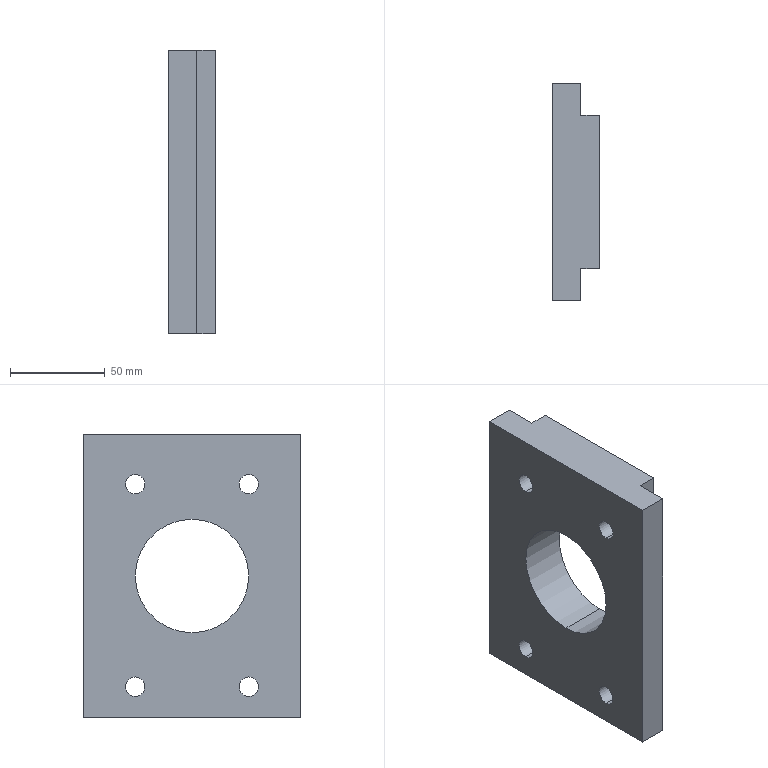Part | SolidWorks | features Extrusion 1, HoleWzd 1, ICE 1 | 1 solid | 20 faces | box 25 x 115 x 150 mm | volume 301393 mm3 | cylinder 10 | plane 10 | commonest cylinder face diameters 10.2 x8 60 x2
STEP:
#1=CARTESIAN_POINT('',(25.,30.,-63.6));
#2=VERTEX_POINT('',#1);
#3=CARTESIAN_POINT('',(25.,30.,-53.4));
#4=VERTEX_POINT('',#3);
#5=CARTESIAN_POINT('',(25.,30.,-58.5));
#6=DIRECTION('',(-1.,0.,0.));
#7=DIRECTION('',(0.,0.,1.));
#8=AXIS2_PLACEMENT_3D('',#5,#6,#7);
#9=CIRCLE('',#8,5.1);
#10=EDGE_CURVE('',#2,#4,#9,.T.);
#11=ORIENTED_EDGE('',*,*,#10,.F.);
#12=CARTESIAN_POINT('',(0.,30.,-63.6));
#13=VERTEX_POINT('',#12);
#14=CARTESIAN_POINT('',(0.,30.,-63.6));
#15=DIRECTION('',(-1.,0.,0.));
#16=VECTOR('',#15,1000.);
#17=LINE('',#14,#16);
#18=EDGE_CURVE('',#2,#13,#17,.T.);
#19=ORIENTED_EDGE('',*,*,#18,.T.);
#20=CARTESIAN_POINT('',(0.,30.,-53.4));
#21=VERTEX_POINT('',#20);
#22=CARTESIAN_POINT('',(0.,30.,-58.5));
#23=DIRECTION('',(-1.,0.,0.));
#24=DIRECTION('',(0.,0.,1.));
#25=AXIS2_PLACEMENT_3D('',#22,#23,#24);
#26=CIRCLE('',#25,5.1);
#27=EDGE_CURVE('',#13,#21,#26,.T.);
#28=ORIENTED_EDGE('',*,*,#27,.T.);
#29=CARTESIAN_POINT('',(0.,30.,-53.4));
#30=DIRECTION('',(-1.,0.,0.));
#31=VECTOR('',#30,1000.);
#32=LINE('',#29,#31);
#33=EDGE_CURVE('',#4,#21,#32,.T.);
#34=ORIENTED_EDGE('',*,*,#33,.F.);
#35=EDGE_LOOP('',(#11,#19,#28,#34));
#36=FACE_OUTER_BOUND('',#35,.T.);
#37=CARTESIAN_POINT('',(0.,30.,-58.5));
#38=DIRECTION('',(-1.,0.,0.));
#39=DIRECTION('',(0.,0.,1.));
#40=AXIS2_PLACEMENT_3D('',#37,#38,#39);
#41=CYLINDRICAL_SURFACE('',#40,5.1);
#42=ADVANCED_FACE('',(#36),#41,.F.);
#43=CARTESIAN_POINT('',(25.,30.,43.4));
#44=VERTEX_POINT('',#43);
#45=CARTESIAN_POINT('',(25.,30.,53.6));
#46=VERTEX_POINT('',#45);
#47=CARTESIAN_POINT('',(25.,30.,48.5));
#48=DIRECTION('',(-1.,0.,0.));
#49=DIRECTION('',(0.,0.,1.));
#50=AXIS2_PLACEMENT_3D('',#47,#48,#49);
#51=CIRCLE('',#50,5.1);
#52=EDGE_CURVE('',#44,#46,#51,.T.);
#53=ORIENTED_EDGE('',*,*,#52,.F.);
#54=CARTESIAN_POINT('',(0.,30.,43.4));
#55=VERTEX_POINT('',#54);
#56=CARTESIAN_POINT('',(0.,30.,43.4));
#57=DIRECTION('',(-1.,0.,0.));
#58=VECTOR('',#57,1000.);
#59=LINE('',#56,#58);
#60=EDGE_CURVE('',#44,#55,#59,.T.);
#61=ORIENTED_EDGE('',*,*,#60,.T.);
#62=CARTESIAN_POINT('',(0.,30.,53.6));
#63=VERTEX_POINT('',#62);
#64=CARTESIAN_POINT('',(0.,30.,48.5));
#65=DIRECTION('',(-1.,0.,0.));
#66=DIRECTION('',(0.,0.,1.));
#67=AXIS2_PLACEMENT_3D('',#64,#65,#66);
#68=CIRCLE('',#67,5.1);
#69=EDGE_CURVE('',#55,#63,#68,.T.);
#70=ORIENTED_EDGE('',*,*,#69,.T.);
#71=CARTESIAN_POINT('',(0.,30.,53.6));
#72=DIRECTION('',(-1.,0.,0.));
#73=VECTOR('',#72,1000.);
#74=LINE('',#71,#73);
#75=EDGE_CURVE('',#46,#63,#74,.T.);
#76=ORIENTED_EDGE('',*,*,#75,.F.);
#77=EDGE_LOOP('',(#53,#61,#70,#76));
#78=FACE_OUTER_BOUND('',#77,.T.);
#79=CARTESIAN_POINT('',(0.,30.,48.5));
#80=DIRECTION('',(-1.,0.,0.));
#81=DIRECTION('',(0.,0.,1.));
#82=AXIS2_PLACEMENT_3D('',#79,#80,#81);
#83=CYLINDRICAL_SURFACE('',#82,5.1);
#84=ADVANCED_FACE('',(#78),#83,.F.);
#85=CARTESIAN_POINT('',(25.,-30.,43.4));
#86=VERTEX_POINT('',#85);
#87=CARTESIAN_POINT('',(25.,-30.,53.6));
#88=VERTEX_POINT('',#87);
#89=CARTESIAN_POINT('',(25.,-30.,48.5));
#90=DIRECTION('',(-1.,0.,0.));
#91=DIRECTION('',(0.,0.,1.));
#92=AXIS2_PLACEMENT_3D('',#89,#90,#91);
#93=CIRCLE('',#92,5.1);
#94=EDGE_CURVE('',#86,#88,#93,.T.);
#95=ORIENTED_EDGE('',*,*,#94,.F.);
#96=CARTESIAN_POINT('',(0.,-30.,43.4));
#97=VERTEX_POINT('',#96);
#98=CARTESIAN_POINT('',(0.,-30.,43.4));
#99=DIRECTION('',(-1.,0.,0.));
#100=VECTOR('',#99,1000.);
#101=LINE('',#98,#100);
#102=EDGE_CURVE('',#86,#97,#101,.T.);
#103=ORIENTED_EDGE('',*,*,#102,.T.);
#104=CARTESIAN_POINT('',(0.,-30.,53.6));
#105=VERTEX_POINT('',#104);
#106=CARTESIAN_POINT('',(0.,-30.,48.5));
#107=DIRECTION('',(-1.,0.,0.));
#108=DIRECTION('',(0.,0.,1.));
#109=AXIS2_PLACEMENT_3D('',#106,#107,#108);
#110=CIRCLE('',#109,5.1);
#111=EDGE_CURVE('',#97,#105,#110,.T.);
#112=ORIENTED_EDGE('',*,*,#111,.T.);
#113=CARTESIAN_POINT('',(0.,-30.,53.6));
#114=DIRECTION('',(-1.,0.,0.));
#115=VECTOR('',#114,1000.);
#116=LINE('',#113,#115);
#117=EDGE_CURVE('',#88,#105,#116,.T.);
#118=ORIENTED_EDGE('',*,*,#117,.F.);
#119=EDGE_LOOP('',(#95,#103,#112,#118));
#120=FACE_OUTER_BOUND('',#119,.T.);
#121=CARTESIAN_POINT('',(0.,-30.,48.5));
#122=DIRECTION('',(-1.,0.,0.));
#123=DIRECTION('',(0.,0.,1.));
#124=AXIS2_PLACEMENT_3D('',#121,#122,#123);
#125=CYLINDRICAL_SURFACE('',#124,5.1);
#126=ADVANCED_FACE('',(#120),#125,.F.);
#127=CARTESIAN_POINT('',(25.,-30.,-63.6));
#128=VERTEX_POINT('',#127);
#129=CARTESIAN_POINT('',(25.,-30.,-53.4));
#130=VERTEX_POINT('',#129);
#131=CARTESIAN_POINT('',(25.,-30.,-58.5));
#132=DIRECTION('',(-1.,0.,0.));
#133=DIRECTION('',(0.,0.,1.));
#134=AXIS2_PLACEMENT_3D('',#131,#132,#133);
#135=CIRCLE('',#134,5.1);
#136=EDGE_CURVE('',#128,#130,#135,.T.);
#137=ORIENTED_EDGE('',*,*,#136,.F.);
#138=CARTESIAN_POINT('',(0.,-30.,-63.6));
#139=VERTEX_POINT('',#138);
#140=CARTESIAN_POINT('',(0.,-30.,-63.6));
#141=DIRECTION('',(-1.,0.,0.));
#142=VECTOR('',#141,1000.);
#143=LINE('',#140,#142);
#144=EDGE_CURVE('',#128,#139,#143,.T.);
#145=ORIENTED_EDGE('',*,*,#144,.T.);
#146=CARTESIAN_POINT('',(0.,-30.,-53.4));
#147=VERTEX_POINT('',#146);
#148=CARTESIAN_POINT('',(0.,-30.,-58.5));
#149=DIRECTION('',(-1.,0.,0.));
#150=DIRECTION('',(0.,0.,1.));
#151=AXIS2_PLACEMENT_3D('',#148,#149,#150);
#152=CIRCLE('',#151,5.1);
#153=EDGE_CURVE('',#139,#147,#152,.T.);
#154=ORIENTED_EDGE('',*,*,#153,.T.);
#155=CARTESIAN_POINT('',(0.,-30.,-53.4));
#156=DIRECTION('',(-1.,0.,0.));
#157=VECTOR('',#156,1000.);
#158=LINE('',#155,#157);
#159=EDGE_CURVE('',#130,#147,#158,.T.);
#160=ORIENTED_EDGE('',*,*,#159,.F.);
#161=EDGE_LOOP('',(#137,#145,#154,#160));
#162=FACE_OUTER_BOUND('',#161,.T.);
#163=CARTESIAN_POINT('',(0.,-30.,-58.5));
#164=DIRECTION('',(-1.,0.,0.));
#165=DIRECTION('',(0.,0.,1.));
#166=AXIS2_PLACEMENT_3D('',#163,#164,#165);
#167=CYLINDRICAL_SURFACE('',#166,5.1);
#168=ADVANCED_FACE('',(#162),#167,.F.);
#169=CARTESIAN_POINT('',(25.,0.,-30.));
#170=VERTEX_POINT('',#169);
#171=CARTESIAN_POINT('',(25.,0.,30.));
#172=VERTEX_POINT('',#171);
#173=CARTESIAN_POINT('',(25.,0.,0.));
#174=DIRECTION('',(-1.,0.,0.));
#175=DIRECTION('',(0.,0.,1.));
#176=AXIS2_PLACEMENT_3D('',#173,#174,#175);
#177=CIRCLE('',#176,30.);
#178=EDGE_CURVE('',#170,#172,#177,.T.);
#179=ORIENTED_EDGE('',*,*,#178,.F.);
#180=CARTESIAN_POINT('',(0.,0.,-30.));
#181=VERTEX_POINT('',#180);
#182=CARTESIAN_POINT('',(210.,0.,-30.));
#183=DIRECTION('',(-1.,0.,0.));
#184=VECTOR('',#183,1000.);
#185=LINE('',#182,#184);
#186=EDGE_CURVE('',#170,#181,#185,.T.);
#187=ORIENTED_EDGE('',*,*,#186,.T.);
#188=CARTESIAN_POINT('',(0.,0.,30.));
#189=VERTEX_POINT('',#188);
#190=CARTESIAN_POINT('',(0.,0.,0.));
#191=DIRECTION('',(-1.,0.,0.));
#192=DIRECTION('',(0.,0.,1.));
#193=AXIS2_PLACEMENT_3D('',#190,#191,#192);
#194=CIRCLE('',#193,30.);
#195=EDGE_CURVE('',#181,#189,#194,.T.);
#196=ORIENTED_EDGE('',*,*,#195,.T.);
#197=CARTESIAN_POINT('',(210.,0.,30.));
#198=DIRECTION('',(-1.,0.,0.));
#199=VECTOR('',#198,1000.);
#200=LINE('',#197,#199);
#201=EDGE_CURVE('',#172,#189,#200,.T.);
#202=ORIENTED_EDGE('',*,*,#201,.F.);
#203=EDGE_LOOP('',(#179,#187,#196,#202));
#204=FACE_OUTER_BOUND('',#203,.T.);
#205=CARTESIAN_POINT('',(210.,0.,0.));
#206=DIRECTION('',(-1.,0.,0.));
#207=DIRECTION('',(0.,0.,1.));
#208=AXIS2_PLACEMENT_3D('',#205,#206,#207);
#209=CYLINDRICAL_SURFACE('',#208,30.);
#210=ADVANCED_FACE('',(#204),#209,.F.);
#211=CARTESIAN_POINT('',(0.,0.,0.));
#212=DIRECTION('',(-1.,0.,0.));
#213=DIRECTION('',(0.,0.,1.));
#214=AXIS2_PLACEMENT_3D('',#211,#212,#213);
#215=CIRCLE('',#214,30.);
#216=EDGE_CURVE('',#189,#181,#215,.T.);
#217=ORIENTED_EDGE('',*,*,#216,.F.);
#218=ORIENTED_EDGE('',*,*,#195,.F.);
#219=EDGE_LOOP('',(#217,#218));
#220=FACE_BOUND('',#219,.T.);
#221=CARTESIAN_POINT('',(0.,57.5,-75.));
#222=VERTEX_POINT('',#221);
#223=CARTESIAN_POINT('',(0.,-57.5,-75.));
#224=VERTEX_POINT('',#223);
#225=CARTESIAN_POINT('',(0.,57.5,-75.));
#226=DIRECTION('',(0.,-1.,0.));
#227=VECTOR('',#226,1000.);
#228=LINE('',#225,#227);
#229=EDGE_CURVE('',#222,#224,#228,.T.);
#230=ORIENTED_EDGE('',*,*,#229,.T.);
#231=CARTESIAN_POINT('',(0.,-57.5,75.));
#232=VERTEX_POINT('',#231);
#233=CARTESIAN_POINT('',(0.,-57.5,75.));
#234=DIRECTION('',(0.,0.,-1.));
#235=VECTOR('',#234,1000.);
#236=LINE('',#233,#235);
#237=EDGE_CURVE('',#232,#224,#236,.T.);
#238=ORIENTED_EDGE('',*,*,#237,.F.);
#239=CARTESIAN_POINT('',(0.,57.5,75.));
#240=VERTEX_POINT('',#239);
#241=CARTESIAN_POINT('',(0.,57.5,75.));
#242=DIRECTION('',(0.,-1.,0.));
#243=VECTOR('',#242,1000.);
#244=LINE('',#241,#243);
#245=EDGE_CURVE('',#240,#232,#244,.T.);
#246=ORIENTED_EDGE('',*,*,#245,.F.);
#247=CARTESIAN_POINT('',(0.,57.5,75.));
#248=DIRECTION('',(0.,0.,-1.));
#249=VECTOR('',#248,1000.);
#250=LINE('',#247,#249);
#251=EDGE_CURVE('',#240,#222,#250,.T.);
#252=ORIENTED_EDGE('',*,*,#251,.T.);
#253=EDGE_LOOP('',(#230,#238,#246,#252));
#254=FACE_OUTER_BOUND('',#253,.T.);
#255=CARTESIAN_POINT('',(0.,-30.,-58.5));
#256=DIRECTION('',(-1.,0.,0.));
#257=DIRECTION('',(0.,0.,1.));
#258=AXIS2_PLACEMENT_3D('',#255,#256,#257);
#259=CIRCLE('',#258,5.1);
#260=EDGE_CURVE('',#147,#139,#259,.T.);
#261=ORIENTED_EDGE('',*,*,#260,.F.);
#262=ORIENTED_EDGE('',*,*,#153,.F.);
#263=EDGE_LOOP('',(#261,#262));
#264=FACE_BOUND('',#263,.T.);
#265=CARTESIAN_POINT('',(0.,-30.,48.5));
#266=DIRECTION('',(-1.,0.,0.));
#267=DIRECTION('',(0.,0.,1.));
#268=AXIS2_PLACEMENT_3D('',#265,#266,#267);
#269=CIRCLE('',#268,5.1);
#270=EDGE_CURVE('',#105,#97,#269,.T.);
#271=ORIENTED_EDGE('',*,*,#270,.F.);
#272=ORIENTED_EDGE('',*,*,#111,.F.);
#273=EDGE_LOOP('',(#271,#272));
#274=FACE_BOUND('',#273,.T.);
#275=CARTESIAN_POINT('',(0.,30.,48.5));
#276=DIRECTION('',(-1.,0.,0.));
#277=DIRECTION('',(0.,0.,1.));
#278=AXIS2_PLACEMENT_3D('',#275,#276,#277);
#279=CIRCLE('',#278,5.1);
#280=EDGE_CURVE('',#63,#55,#279,.T.);
#281=ORIENTED_EDGE('',*,*,#280,.F.);
#282=ORIENTED_EDGE('',*,*,#69,.F.);
#283=EDGE_LOOP('',(#281,#282));
#284=FACE_BOUND('',#283,.T.);
#285=CARTESIAN_POINT('',(0.,30.,-58.5));
#286=DIRECTION('',(-1.,0.,0.));
#287=DIRECTION('',(0.,0.,1.));
#288=AXIS2_PLACEMENT_3D('',#285,#286,#287);
#289=CIRCLE('',#288,5.1);
#290=EDGE_CURVE('',#21,#13,#289,.T.);
#291=ORIENTED_EDGE('',*,*,#290,.F.);
#292=ORIENTED_EDGE('',*,*,#27,.F.);
#293=EDGE_LOOP('',(#291,#292));
#294=FACE_BOUND('',#293,.T.);
#295=CARTESIAN_POINT('',(0.,57.5,75.));
#296=DIRECTION('',(1.,0.,0.));
#297=DIRECTION('',(0.,0.,-1.));
#298=AXIS2_PLACEMENT_3D('',#295,#296,#297);
#299=PLANE('',#298);
#300=ADVANCED_FACE('',(#220,#254,#264,#274,#284,#294),#299,.F.);
#301=CARTESIAN_POINT('',(25.,40.5,-75.));
#302=VERTEX_POINT('',#301);
#303=CARTESIAN_POINT('',(15.,40.5,-75.));
#304=VERTEX_POINT('',#303);
#305=CARTESIAN_POINT('',(15.,40.5,-75.));
#306=DIRECTION('',(-1.,0.,0.));
#307=VECTOR('',#306,1000.);
#308=LINE('',#305,#307);
#309=EDGE_CURVE('',#302,#304,#308,.T.);
#310=ORIENTED_EDGE('',*,*,#309,.T.);
#311=CARTESIAN_POINT('',(15.,40.5,75.));
#312=VERTEX_POINT('',#311);
#313=CARTESIAN_POINT('',(15.,40.5,75.));
#314=DIRECTION('',(0.,0.,-1.));
#315=VECTOR('',#314,1000.);
#316=LINE('',#313,#315);
#317=EDGE_CURVE('',#312,#304,#316,.T.);
#318=ORIENTED_EDGE('',*,*,#317,.F.);
#319=CARTESIAN_POINT('',(25.,40.5,75.));
#320=VERTEX_POINT('',#319);
#321=CARTESIAN_POINT('',(15.,40.5,75.));
#322=DIRECTION('',(-1.,0.,0.));
#323=VECTOR('',#322,1000.);
#324=LINE('',#321,#323);
#325=EDGE_CURVE('',#320,#312,#324,.T.);
#326=ORIENTED_EDGE('',*,*,#325,.F.);
#327=CARTESIAN_POINT('',(25.,40.5,75.));
#328=DIRECTION('',(0.,0.,-1.));
#329=VECTOR('',#328,1000.);
#330=LINE('',#327,#329);
#331=EDGE_CURVE('',#320,#302,#330,.T.);
#332=ORIENTED_EDGE('',*,*,#331,.T.);
#333=EDGE_LOOP('',(#310,#318,#326,#332));
#334=FACE_OUTER_BOUND('',#333,.T.);
#335=CARTESIAN_POINT('',(15.,40.5,75.));
#336=DIRECTION('',(0.,-1.,0.));
#337=DIRECTION('',(0.,0.,-1.));
#338=AXIS2_PLACEMENT_3D('',#335,#336,#337);
#339=PLANE('',#338);
#340=ADVANCED_FACE('',(#334),#339,.F.);
#341=CARTESIAN_POINT('',(15.,57.5,-75.));
#342=VERTEX_POINT('',#341);
#343=CARTESIAN_POINT('',(15.,57.5,-75.));
#344=DIRECTION('',(0.,1.,0.));
#345=VECTOR('',#344,1000.);
#346=LINE('',#343,#345);
#347=EDGE_CURVE('',#304,#342,#346,.T.);
#348=ORIENTED_EDGE('',*,*,#347,.T.);
#349=CARTESIAN_POINT('',(15.,57.5,75.));
#350=VERTEX_POINT('',#349);
#351=CARTESIAN_POINT('',(15.,57.5,75.));
#352=DIRECTION('',(0.,0.,-1.));
#353=VECTOR('',#352,1000.);
#354=LINE('',#351,#353);
#355=EDGE_CURVE('',#350,#342,#354,.T.);
#356=ORIENTED_EDGE('',*,*,#355,.F.);
#357=CARTESIAN_POINT('',(15.,57.5,75.));
#358=DIRECTION('',(0.,1.,0.));
#359=VECTOR('',#358,1000.);
#360=LINE('',#357,#359);
#361=EDGE_CURVE('',#312,#350,#360,.T.);
#362=ORIENTED_EDGE('',*,*,#361,.F.);
#363=ORIENTED_EDGE('',*,*,#317,.T.);
#364=EDGE_LOOP('',(#348,#356,#362,#363));
#365=FACE_OUTER_BOUND('',#364,.T.);
#366=CARTESIAN_POINT('',(15.,57.5,75.));
#367=DIRECTION('',(-1.,0.,0.));
#368=DIRECTION('',(0.,0.,1.));
#369=AXIS2_PLACEMENT_3D('',#366,#367,#368);
#370=PLANE('',#369);
#371=ADVANCED_FACE('',(#365),#370,.F.);
#372=CARTESIAN_POINT('',(0.,57.5,-75.));
#373=DIRECTION('',(-1.,0.,0.));
#374=VECTOR('',#373,1000.);
#375=LINE('',#372,#374);
#376=EDGE_CURVE('',#342,#222,#375,.T.);
#377=ORIENTED_EDGE('',*,*,#376,.T.);
#378=ORIENTED_EDGE('',*,*,#251,.F.);
#379=CARTESIAN_POINT('',(0.,57.5,75.));
#380=DIRECTION('',(-1.,0.,0.));
#381=VECTOR('',#380,1000.);
#382=LINE('',#379,#381);
#383=EDGE_CURVE('',#350,#240,#382,.T.);
#384=ORIENTED_EDGE('',*,*,#383,.F.);
#385=ORIENTED_EDGE('',*,*,#355,.T.);
#386=EDGE_LOOP('',(#377,#378,#384,#385));
#387=FACE_OUTER_BOUND('',#386,.T.);
#388=CARTESIAN_POINT('',(0.,57.5,75.));
#389=DIRECTION('',(0.,-1.,0.));
#390=DIRECTION('',(0.,0.,-1.));
#391=AXIS2_PLACEMENT_3D('',#388,#389,#390);
#392=PLANE('',#391);
#393=ADVANCED_FACE('',(#387),#392,.F.);
#394=CARTESIAN_POINT('',(15.,-57.5,-75.));
#395=VERTEX_POINT('',#394);
#396=CARTESIAN_POINT('',(0.,-57.5,-75.));
#397=DIRECTION('',(1.,0.,0.));
#398=VECTOR('',#397,1000.);
#399=LINE('',#396,#398);
#400=EDGE_CURVE('',#224,#395,#399,.T.);
#401=ORIENTED_EDGE('',*,*,#400,.T.);
#402=CARTESIAN_POINT('',(15.,-57.5,75.));
#403=VERTEX_POINT('',#402);
#404=CARTESIAN_POINT('',(15.,-57.5,75.));
#405=DIRECTION('',(0.,0.,-1.));
#406=VECTOR('',#405,1000.);
#407=LINE('',#404,#406);
#408=EDGE_CURVE('',#403,#395,#407,.T.);
#409=ORIENTED_EDGE('',*,*,#408,.F.);
#410=CARTESIAN_POINT('',(0.,-57.5,75.));
#411=DIRECTION('',(1.,0.,0.));
#412=VECTOR('',#411,1000.);
#413=LINE('',#410,#412);
#414=EDGE_CURVE('',#232,#403,#413,.T.);
#415=ORIENTED_EDGE('',*,*,#414,.F.);
#416=ORIENTED_EDGE('',*,*,#237,.T.);
#417=EDGE_LOOP('',(#401,#409,#415,#416));
#418=FACE_OUTER_BOUND('',#417,.T.);
#419=CARTESIAN_POINT('',(0.,-57.5,75.));
#420=DIRECTION('',(0.,1.,0.));
#421=DIRECTION('',(0.,0.,1.));
#422=AXIS2_PLACEMENT_3D('',#419,#420,#421);
#423=PLANE('',#422);
#424=ADVANCED_FACE('',(#418),#423,.F.);
#425=CARTESIAN_POINT('',(15.,-40.5,-75.));
#426=VERTEX_POINT('',#425);
#427=CARTESIAN_POINT('',(15.,-57.5,-75.));
#428=DIRECTION('',(0.,1.,0.));
#429=VECTOR('',#428,1000.);
#430=LINE('',#427,#429);
#431=EDGE_CURVE('',#395,#426,#430,.T.);
#432=ORIENTED_EDGE('',*,*,#431,.T.);
#433=CARTESIAN_POINT('',(15.,-40.5,75.));
#434=VERTEX_POINT('',#433);
#435=CARTESIAN_POINT('',(15.,-40.5,75.));
#436=DIRECTION('',(0.,0.,-1.));
#437=VECTOR('',#436,1000.);
#438=LINE('',#435,#437);
#439=EDGE_CURVE('',#434,#426,#438,.T.);
#440=ORIENTED_EDGE('',*,*,#439,.F.);
#441=CARTESIAN_POINT('',(15.,-57.5,75.));
#442=DIRECTION('',(0.,1.,0.));
#443=VECTOR('',#442,1000.);
#444=LINE('',#441,#443);
#445=EDGE_CURVE('',#403,#434,#444,.T.);
#446=ORIENTED_EDGE('',*,*,#445,.F.);
#447=ORIENTED_EDGE('',*,*,#408,.T.);
#448=EDGE_LOOP('',(#432,#440,#446,#447));
#449=FACE_OUTER_BOUND('',#448,.T.);
#450=CARTESIAN_POINT('',(15.,-57.5,75.));
#451=DIRECTION('',(-1.,0.,0.));
#452=DIRECTION('',(0.,0.,1.));
#453=AXIS2_PLACEMENT_3D('',#450,#451,#452);
#454=PLANE('',#453);
#455=ADVANCED_FACE('',(#449),#454,.F.);
#456=CARTESIAN_POINT('',(25.,-40.5,-75.));
#457=VERTEX_POINT('',#456);
#458=CARTESIAN_POINT('',(15.,-40.5,-75.));
#459=DIRECTION('',(1.,0.,0.));
#460=VECTOR('',#459,1000.);
#461=LINE('',#458,#460);
#462=EDGE_CURVE('',#426,#457,#461,.T.);
#463=ORIENTED_EDGE('',*,*,#462,.T.);
#464=CARTESIAN_POINT('',(25.,-40.5,75.));
#465=VERTEX_POINT('',#464);
#466=CARTESIAN_POINT('',(25.,-40.5,75.));
#467=DIRECTION('',(0.,0.,-1.));
#468=VECTOR('',#467,1000.);
#469=LINE('',#466,#468);
#470=EDGE_CURVE('',#465,#457,#469,.T.);
#471=ORIENTED_EDGE('',*,*,#470,.F.);
#472=CARTESIAN_POINT('',(15.,-40.5,75.));
#473=DIRECTION('',(1.,0.,0.));
#474=VECTOR('',#473,1000.);
#475=LINE('',#472,#474);
#476=EDGE_CURVE('',#434,#465,#475,.T.);
#477=ORIENTED_EDGE('',*,*,#476,.F.);
#478=ORIENTED_EDGE('',*,*,#439,.T.);
#479=EDGE_LOOP('',(#463,#471,#477,#478));
#480=FACE_OUTER_BOUND('',#479,.T.);
#481=CARTESIAN_POINT('',(15.,-40.5,75.));
#482=DIRECTION('',(0.,1.,0.));
#483=DIRECTION('',(0.,0.,1.));
#484=AXIS2_PLACEMENT_3D('',#481,#482,#483);
#485=PLANE('',#484);
#486=ADVANCED_FACE('',(#480),#485,.F.);
#487=CARTESIAN_POINT('',(25.,30.,-58.5));
#488=DIRECTION('',(-1.,0.,0.));
#489=DIRECTION('',(0.,0.,1.));
#490=AXIS2_PLACEMENT_3D('',#487,#488,#489);
#491=CIRCLE('',#490,5.1);
#492=EDGE_CURVE('',#4,#2,#491,.T.);
#493=ORIENTED_EDGE('',*,*,#492,.T.);
#494=ORIENTED_EDGE('',*,*,#10,.T.);
#495=EDGE_LOOP('',(#493,#494));
#496=FACE_BOUND('',#495,.T.);
#497=CARTESIAN_POINT('',(25.,30.,48.5));
#498=DIRECTION('',(-1.,0.,0.));
#499=DIRECTION('',(0.,0.,1.));
#500=AXIS2_PLACEMENT_3D('',#497,#498,#499);
#501=CIRCLE('',#500,5.1);
#502=EDGE_CURVE('',#46,#44,#501,.T.);
#503=ORIENTED_EDGE('',*,*,#502,.T.);
#504=ORIENTED_EDGE('',*,*,#52,.T.);
#505=EDGE_LOOP('',(#503,#504));
#506=FACE_BOUND('',#505,.T.);
#507=CARTESIAN_POINT('',(25.,-30.,48.5));
#508=DIRECTION('',(-1.,0.,0.));
#509=DIRECTION('',(0.,0.,1.));
#510=AXIS2_PLACEMENT_3D('',#507,#508,#509);
#511=CIRCLE('',#510,5.1);
#512=EDGE_CURVE('',#88,#86,#511,.T.);
#513=ORIENTED_EDGE('',*,*,#512,.T.);
#514=ORIENTED_EDGE('',*,*,#94,.T.);
#515=EDGE_LOOP('',(#513,#514));
#516=FACE_BOUND('',#515,.T.);
#517=CARTESIAN_POINT('',(25.,-30.,-58.5));
#518=DIRECTION('',(-1.,0.,0.));
#519=DIRECTION('',(0.,0.,1.));
#520=AXIS2_PLACEMENT_3D('',#517,#518,#519);
#521=CIRCLE('',#520,5.1);
#522=EDGE_CURVE('',#130,#128,#521,.T.);
#523=ORIENTED_EDGE('',*,*,#522,.T.);
#524=ORIENTED_EDGE('',*,*,#136,.T.);
#525=EDGE_LOOP('',(#523,#524));
#526=FACE_BOUND('',#525,.T.);
#527=CARTESIAN_POINT('',(25.,0.,0.));
#528=DIRECTION('',(-1.,0.,0.));
#529=DIRECTION('',(0.,0.,1.));
#530=AXIS2_PLACEMENT_3D('',#527,#528,#529);
#531=CIRCLE('',#530,30.);
#532=EDGE_CURVE('',#172,#170,#531,.T.);
#533=ORIENTED_EDGE('',*,*,#532,.T.);
#534=ORIENTED_EDGE('',*,*,#178,.T.);
#535=EDGE_LOOP('',(#533,#534));
#536=FACE_BOUND('',#535,.T.);
#537=CARTESIAN_POINT('',(25.,-40.5,-75.));
#538=DIRECTION('',(0.,1.,0.));
#539=VECTOR('',#538,1000.);
#540=LINE('',#537,#539);
#541=EDGE_CURVE('',#457,#302,#540,.T.);
#542=ORIENTED_EDGE('',*,*,#541,.T.);
#543=ORIENTED_EDGE('',*,*,#331,.F.);
#544=CARTESIAN_POINT('',(25.,-40.5,75.));
#545=DIRECTION('',(0.,1.,0.));
#546=VECTOR('',#545,1000.);
#547=LINE('',#544,#546);
#548=EDGE_CURVE('',#465,#320,#547,.T.);
#549=ORIENTED_EDGE('',*,*,#548,.F.);
#550=ORIENTED_EDGE('',*,*,#470,.T.);
#551=EDGE_LOOP('',(#542,#543,#549,#550));
#552=FACE_OUTER_BOUND('',#551,.T.);
#553=CARTESIAN_POINT('',(25.,-40.5,75.));
#554=DIRECTION('',(-1.,0.,0.));
#555=DIRECTION('',(0.,0.,1.));
#556=AXIS2_PLACEMENT_3D('',#553,#554,#555);
#557=PLANE('',#556);
#558=ADVANCED_FACE('',(#496,#506,#516,#526,#536,#552),#557,.F.);
#559=ORIENTED_EDGE('',*,*,#325,.T.);
#560=ORIENTED_EDGE('',*,*,#361,.T.);
#561=ORIENTED_EDGE('',*,*,#383,.T.);
#562=ORIENTED_EDGE('',*,*,#245,.T.);
#563=ORIENTED_EDGE('',*,*,#414,.T.);
#564=ORIENTED_EDGE('',*,*,#445,.T.);
#565=ORIENTED_EDGE('',*,*,#476,.T.);
#566=ORIENTED_EDGE('',*,*,#548,.T.);
#567=EDGE_LOOP('',(#559,#560,#561,#562,#563,#564,#565,#566));
#568=FACE_OUTER_BOUND('',#567,.T.);
#569=CARTESIAN_POINT('',(0.,0.,75.));
#570=DIRECTION('',(0.,0.,1.));
#571=DIRECTION('',(1.,0.,0.));
#572=AXIS2_PLACEMENT_3D('',#569,#570,#571);
#573=PLANE('',#572);
#574=ADVANCED_FACE('',(#568),#573,.T.);
#575=ORIENTED_EDGE('',*,*,#309,.F.);
#576=ORIENTED_EDGE('',*,*,#541,.F.);
#577=ORIENTED_EDGE('',*,*,#462,.F.);
#578=ORIENTED_EDGE('',*,*,#431,.F.);
#579=ORIENTED_EDGE('',*,*,#400,.F.);
#580=ORIENTED_EDGE('',*,*,#229,.F.);
#581=ORIENTED_EDGE('',*,*,#376,.F.);
#582=ORIENTED_EDGE('',*,*,#347,.F.);
#583=EDGE_LOOP('',(#575,#576,#577,#578,#579,#580,#581,#582));
#584=FACE_OUTER_BOUND('',#583,.T.);
#585=CARTESIAN_POINT('',(0.,0.,-75.));
#586=DIRECTION('',(0.,0.,1.));
#587=DIRECTION('',(1.,0.,0.));
#588=AXIS2_PLACEMENT_3D('',#585,#586,#587);
#589=PLANE('',#588);
#590=ADVANCED_FACE('',(#584),#589,.F.);
#591=ORIENTED_EDGE('',*,*,#186,.F.);
#592=ORIENTED_EDGE('',*,*,#532,.F.);
#593=ORIENTED_EDGE('',*,*,#201,.T.);
#594=ORIENTED_EDGE('',*,*,#216,.T.);
#595=EDGE_LOOP('',(#591,#592,#593,#594));
#596=FACE_OUTER_BOUND('',#595,.T.);
#597=CARTESIAN_POINT('',(210.,0.,0.));
#598=DIRECTION('',(-1.,0.,0.));
#599=DIRECTION('',(0.,0.,1.));
#600=AXIS2_PLACEMENT_3D('',#597,#598,#599);
#601=CYLINDRICAL_SURFACE('',#600,30.);
#602=ADVANCED_FACE('',(#596),#601,.F.);
#603=ORIENTED_EDGE('',*,*,#144,.F.);
#604=ORIENTED_EDGE('',*,*,#522,.F.);
#605=ORIENTED_EDGE('',*,*,#159,.T.);
#606=ORIENTED_EDGE('',*,*,#260,.T.);
#607=EDGE_LOOP('',(#603,#604,#605,#606));
#608=FACE_OUTER_BOUND('',#607,.T.);
#609=CARTESIAN_POINT('',(0.,-30.,-58.5));
#610=DIRECTION('',(-1.,0.,0.));
#611=DIRECTION('',(0.,0.,1.));
#612=AXIS2_PLACEMENT_3D('',#609,#610,#611);
#613=CYLINDRICAL_SURFACE('',#612,5.1);
#614=ADVANCED_FACE('',(#608),#613,.F.);
#615=ORIENTED_EDGE('',*,*,#102,.F.);
#616=ORIENTED_EDGE('',*,*,#512,.F.);
#617=ORIENTED_EDGE('',*,*,#117,.T.);
#618=ORIENTED_EDGE('',*,*,#270,.T.);
#619=EDGE_LOOP('',(#615,#616,#617,#618));
#620=FACE_OUTER_BOUND('',#619,.T.);
#621=CARTESIAN_POINT('',(0.,-30.,48.5));
#622=DIRECTION('',(-1.,0.,0.));
#623=DIRECTION('',(0.,0.,1.));
#624=AXIS2_PLACEMENT_3D('',#621,#622,#623);
#625=CYLINDRICAL_SURFACE('',#624,5.1);
#626=ADVANCED_FACE('',(#620),#625,.F.);
#627=ORIENTED_EDGE('',*,*,#60,.F.);
#628=ORIENTED_EDGE('',*,*,#502,.F.);
#629=ORIENTED_EDGE('',*,*,#75,.T.);
#630=ORIENTED_EDGE('',*,*,#280,.T.);
#631=EDGE_LOOP('',(#627,#628,#629,#630));
#632=FACE_OUTER_BOUND('',#631,.T.);
#633=CARTESIAN_POINT('',(0.,30.,48.5));
#634=DIRECTION('',(-1.,0.,0.));
#635=DIRECTION('',(0.,0.,1.));
#636=AXIS2_PLACEMENT_3D('',#633,#634,#635);
#637=CYLINDRICAL_SURFACE('',#636,5.1);
#638=ADVANCED_FACE('',(#632),#637,.F.);
#639=ORIENTED_EDGE('',*,*,#18,.F.);
#640=ORIENTED_EDGE('',*,*,#492,.F.);
#641=ORIENTED_EDGE('',*,*,#33,.T.);
#642=ORIENTED_EDGE('',*,*,#290,.T.);
#643=EDGE_LOOP('',(#639,#640,#641,#642));
#644=FACE_OUTER_BOUND('',#643,.T.);
#645=CARTESIAN_POINT('',(0.,30.,-58.5));
#646=DIRECTION('',(-1.,0.,0.));
#647=DIRECTION('',(0.,0.,1.));
#648=AXIS2_PLACEMENT_3D('',#645,#646,#647);
#649=CYLINDRICAL_SURFACE('',#648,5.1);
#650=ADVANCED_FACE('',(#644),#649,.F.);
#651=CLOSED_SHELL('',(#42,#84,#126,#168,#210,#300,#340,#371,#393,#424,#455,#486,#558,#574,#590,#602,#614,#626,#638,#650));
#652=MANIFOLD_SOLID_BREP('',#651);
#653=CARTESIAN_POINT('',(0.,0.,0.));
#654=DIRECTION('',(0.,0.,1.));
#655=DIRECTION('',(1.,0.,0.));
#656=AXIS2_PLACEMENT_3D('',#653,#654,#655);
#657=(LENGTH_UNIT()NAMED_UNIT(*)SI_UNIT(.MILLI.,.METRE.));
#658=UNCERTAINTY_MEASURE_WITH_UNIT(LENGTH_MEASURE(0.00001),#657,'','');
#659=(NAMED_UNIT(*)PLANE_ANGLE_UNIT()SI_UNIT($,.RADIAN.));
#660=(NAMED_UNIT(*)SI_UNIT($,.STERADIAN.)SOLID_ANGLE_UNIT());
#661=(GEOMETRIC_REPRESENTATION_CONTEXT(3)GLOBAL_UNCERTAINTY_ASSIGNED_CONTEXT((#658))GLOBAL_UNIT_ASSIGNED_CONTEXT((#657,#659,#660))REPRESENTATION_CONTEXT('',''));
#662=ADVANCED_BREP_SHAPE_REPRESENTATION('',(#652,#656),#661);